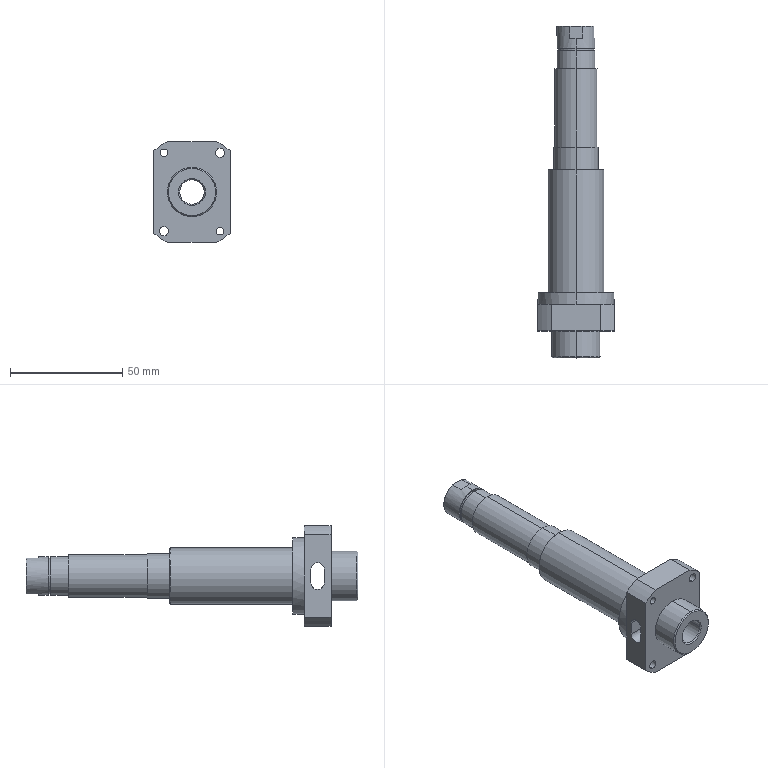Part | SolidWorks | features ICE 6, Chamfer 2, HoleWzd 1, Revolution 1 | 1 solid | 71 faces | box 34 x 148 x 45 mm | volume 55007 mm3 | cylinder 35 | plane 25 | cone 11 | commonest cylinder face diameters 3.3 x4 4 x4 11 x4 17 x4 50 x4 6 x3